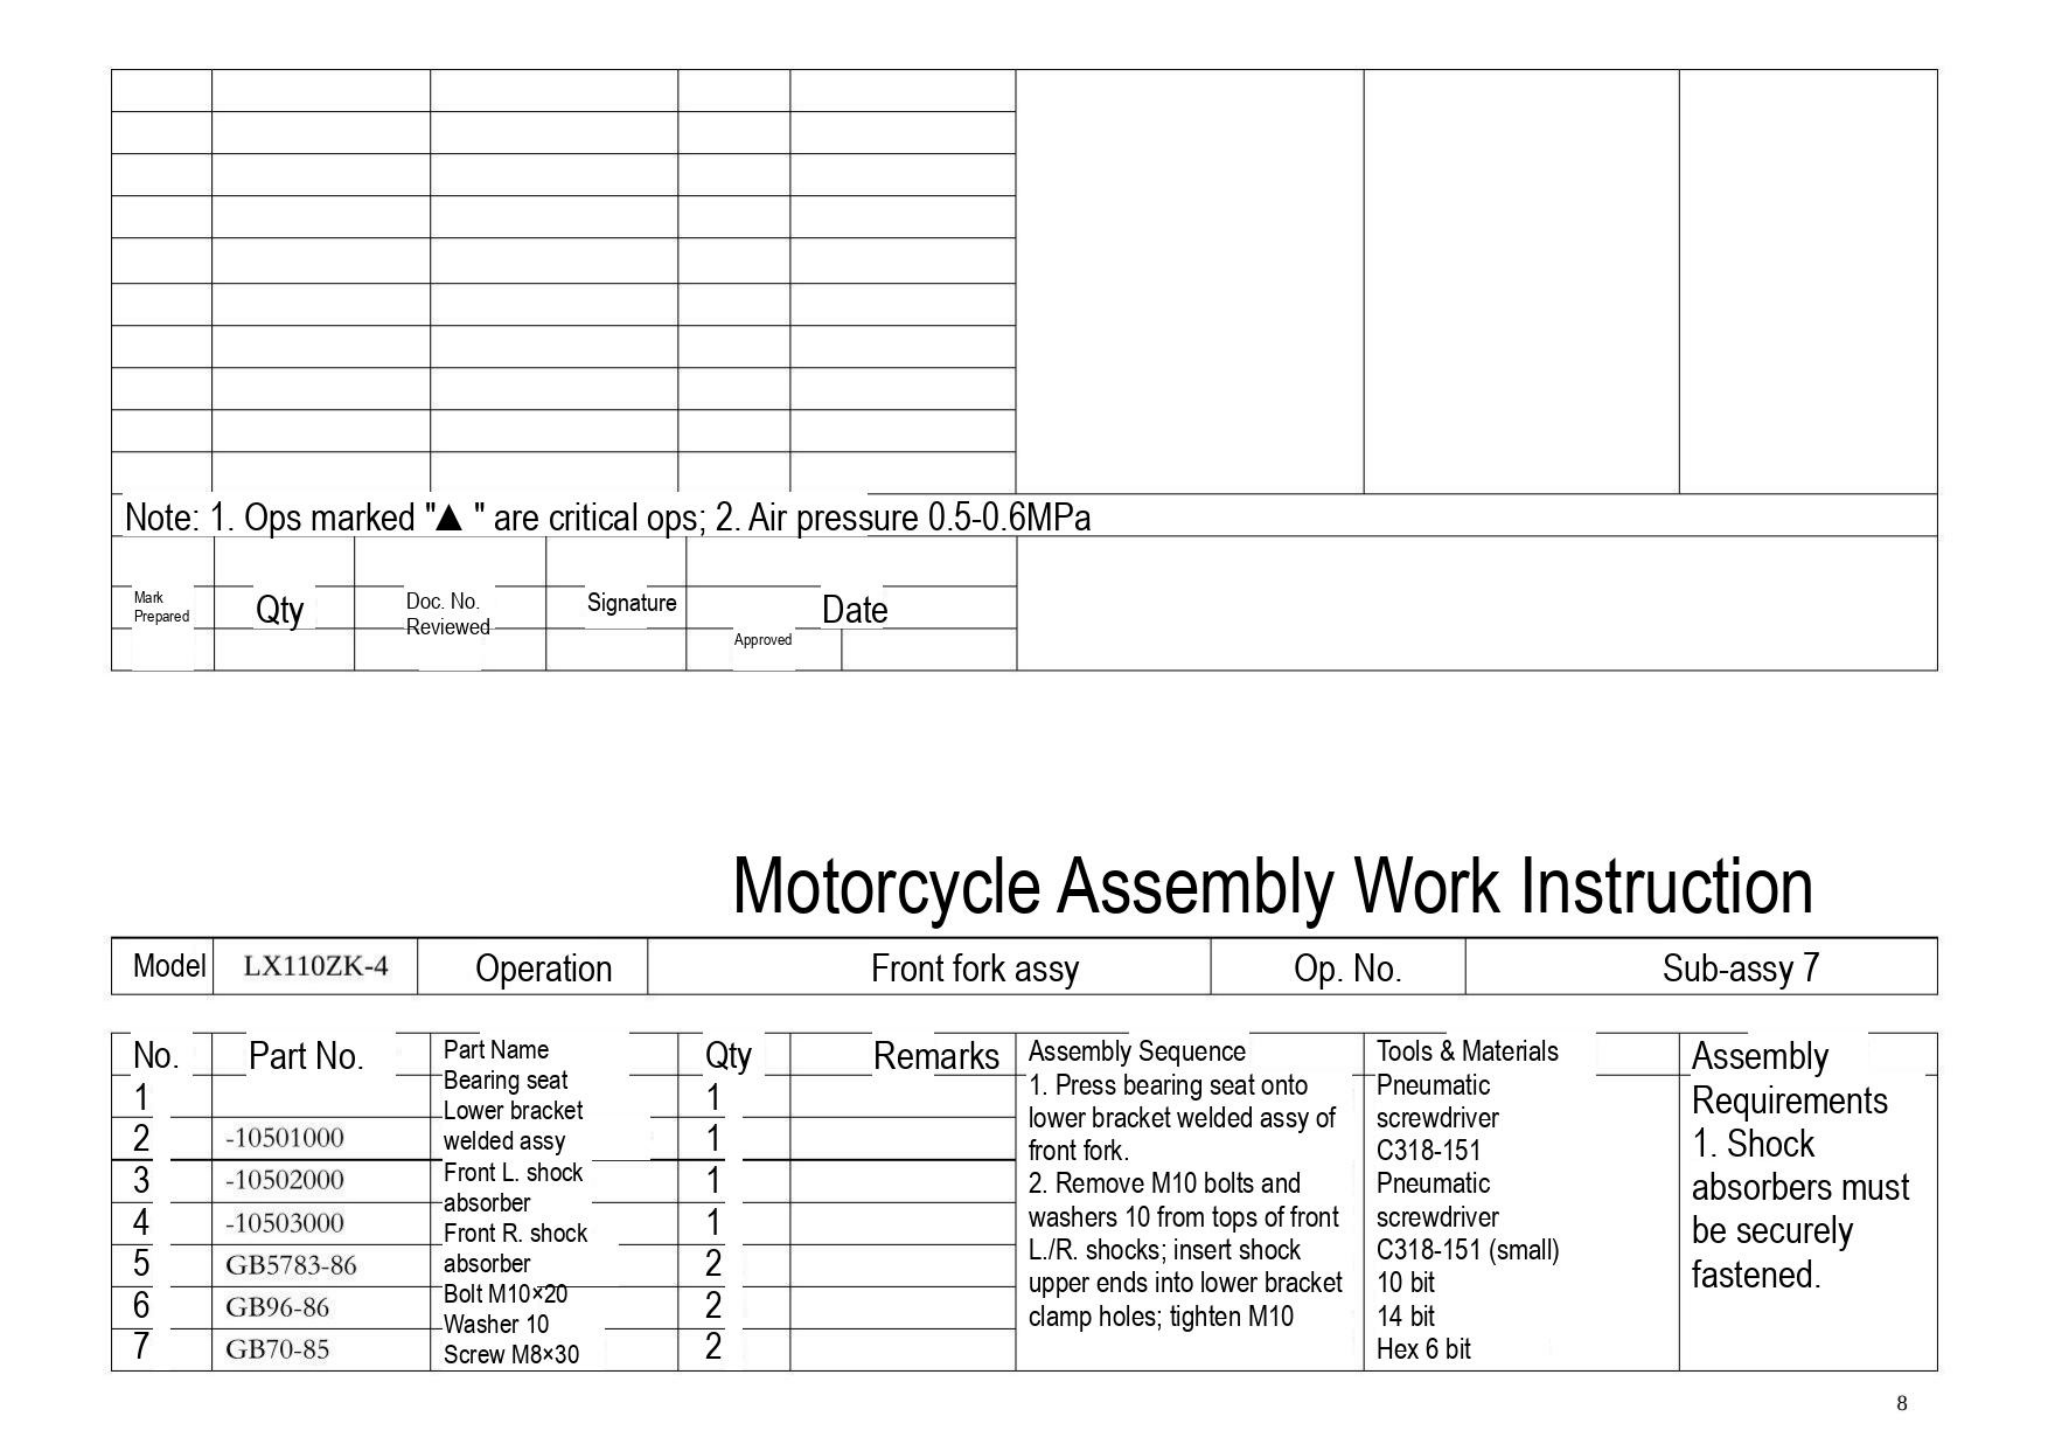Note: 1. Ops marked "▲ " are critical ops; 2. Air pressure 0.5-0.6MPa

| Mark Prepared | Qty | Doc. No. Reviewed | Signature | Approved | Date |
|---|---|---|---|---|---|
| | | | | | |

# Motorcycle Assembly Work Instruction

| Model | LX110ZK-4 | Operation | Front fork assy | Op. No. | Sub-assy 7 |
|---|---|---|---|---|---|

| No. | Part No. | Part Name | Qty | Remarks | Assembly Sequence | Tools & Materials | Assembly Requirements |
|---|---|---|---|---|---|---|---|
| 1 | | Bearing seat | 1 | | 1. Press bearing seat onto lower bracket welded assy of front fork.<br>2. Remove M10 bolts and washers 10 from tops of front L./R. shocks; insert shock upper ends into lower bracket clamp holes; tighten M10 | Pneumatic screwdriver C318-151<br>Pneumatic screwdriver C318-151 (small)<br>10 bit<br>14 bit<br>Hex 6 bit | 1. Shock absorbers must be securely fastened. |
| 2 | -10501000 | Lower bracket welded assy | 1 | | | | |
| 3 | -10502000 | Front L. shock absorber | 1 | | | | |
| 4 | -10503000 | Front R. shock absorber | 1 | | | | |
| 5 | GB5783-86 | Bolt M10×20 | 2 | | | | |
| 6 | GB96-86 | Washer 10 | 2 | | | | |
| 7 | GB70-85 | Screw M8×30 | 2 | | | | |

8
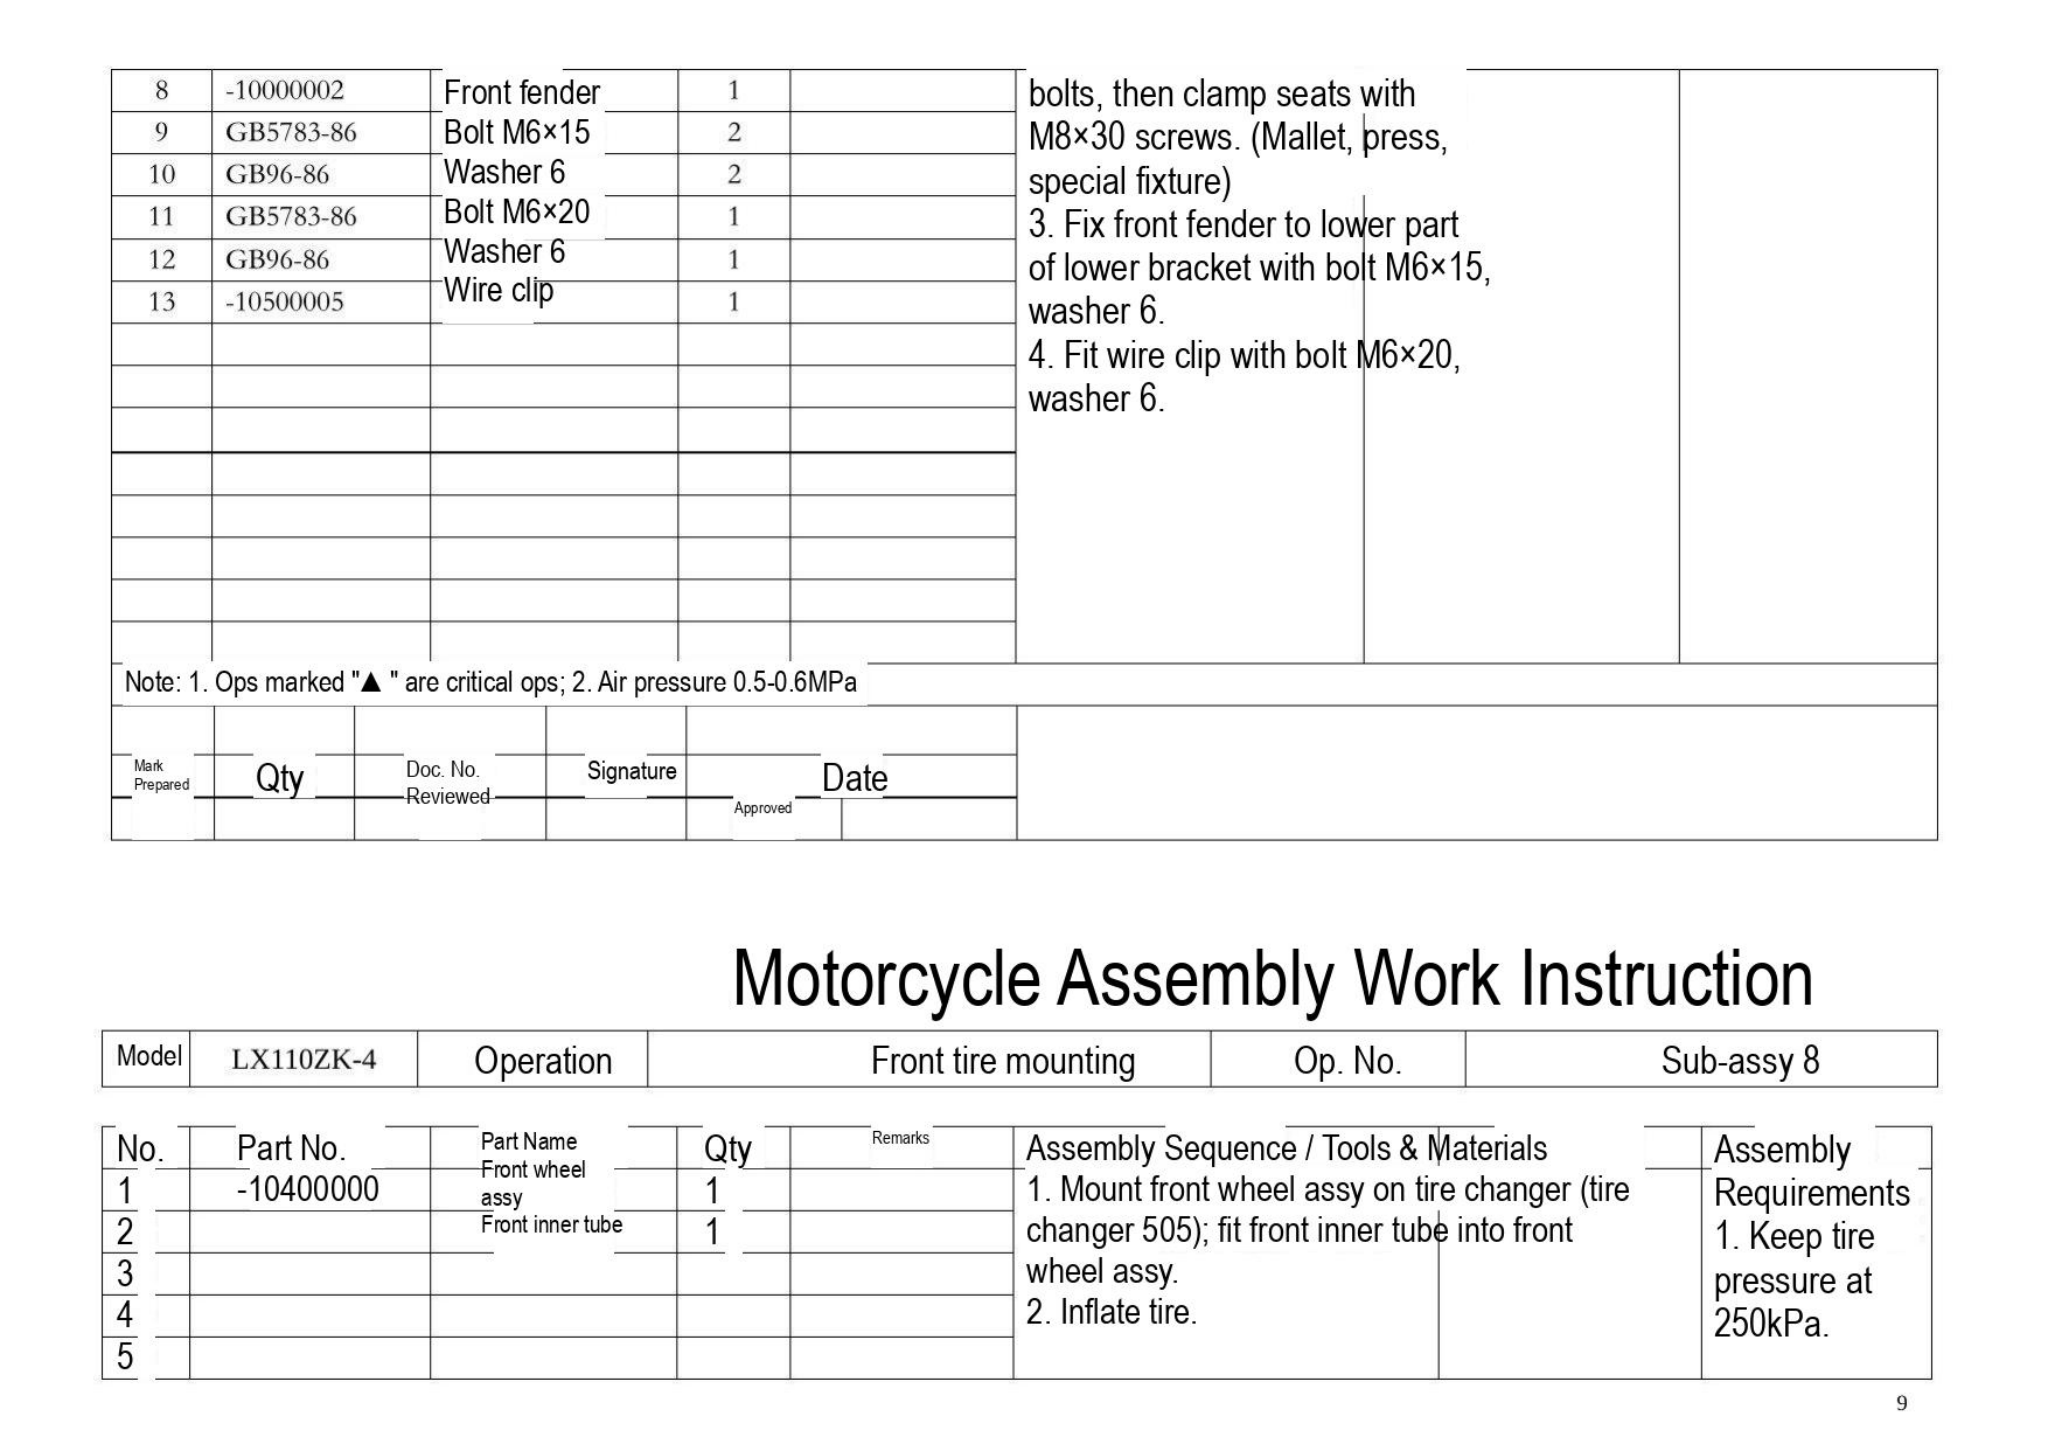| 8 | -10000002 | Front fender | 1 | |
|---|---|---|---|---|
| 9 | GB5783-86 | Bolt M6×15 | 2 | |
| 10 | GB96-86 | Washer 6 | 2 | |
| 11 | GB5783-86 | Bolt M6×20 | 1 | |
| 12 | GB96-86 | Washer 6 | 1 | |
| 13 | -10500005 | Wire clip | 1 | |

bolts, then clamp seats with M8×30 screws. (Mallet, press, special fixture)
3. Fix front fender to lower part of lower bracket with bolt M6×15, washer 6.
4. Fit wire clip with bolt M6×20, washer 6.

Note: 1. Ops marked "▲ " are critical ops; 2. Air pressure 0.5-0.6MPa

| Mark | Qty | Doc. No. | Signature | Date |
|---|---|---|---|---|
| Prepared | | Reviewed | | Approved |

Motorcycle Assembly Work Instruction

| Model | LX110ZK-4 | Operation | Front tire mounting | Op. No. | Sub-assy 8 |
|---|---|---|---|---|---|

| No. | Part No. | Part Name | Qty | Remarks |
|---|---|---|---|---|
| 1 | -10400000 | Front wheel assy | 1 | |
| 2 | | Front inner tube | 1 | |
| 3 | | | | |
| 4 | | | | |
| 5 | | | | |

Assembly Sequence / Tools & Materials
1. Mount front wheel assy on tire changer (tire changer 505); fit front inner tube into front wheel assy.
2. Inflate tire.

Assembly Requirements
1. Keep tire pressure at 250kPa.

9
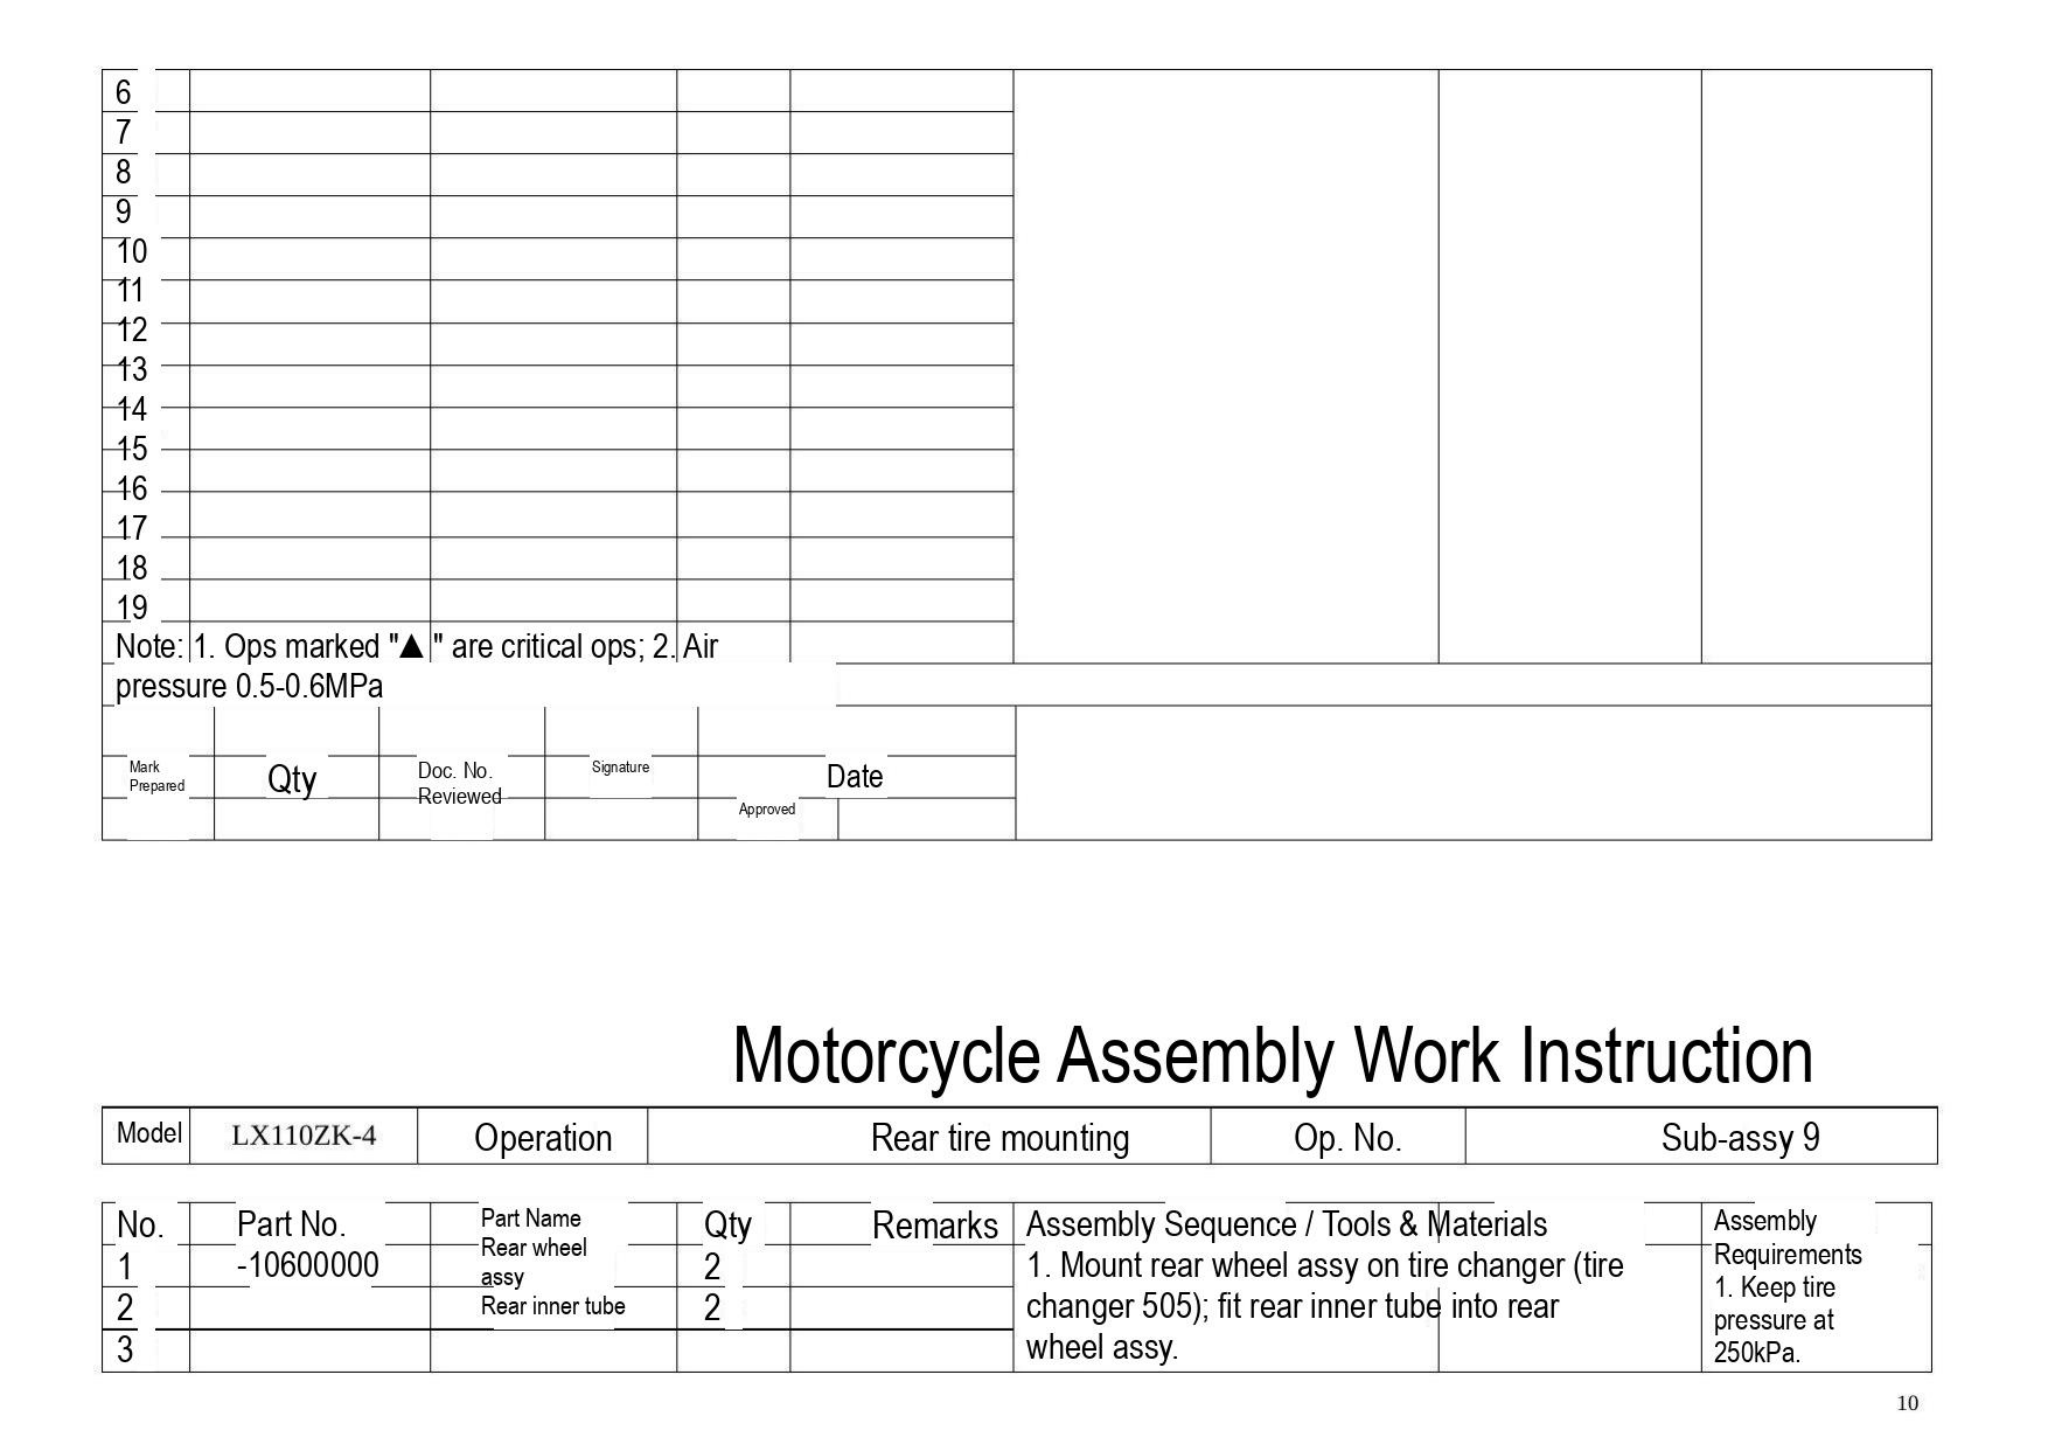| 6 | | | | |
|---|---|---|---|---|
| 7 | | | | |
| 8 | | | | |
| 9 | | | | |
| 10 | | | | |
| 11 | | | | |
| 12 | | | | |
| 13 | | | | |
| 14 | | | | |
| 15 | | | | |
| 16 | | | | |
| 17 | | | | |
| 18 | | | | |
| 19 | | | | |

Note: 1. Ops marked "▲" are critical ops; 2. Air pressure 0.5-0.6MPa

| Mark Prepared | Qty | Doc. No. Reviewed | Signature | Approved | Date |
|---|---|---|---|---|---|
| | | | | | |

# Motorcycle Assembly Work Instruction

| Model | LX110ZK-4 | Operation | Rear tire mounting | Op. No. | Sub-assy 9 |
|---|---|---|---|---|---|

| No. | Part No. | Part Name | Qty | Remarks | Assembly Sequence / Tools & Materials | Assembly Requirements |
|---|---|---|---|---|---|---|
| 1 | -10600000 | Rear wheel assy | 2 | | 1. Mount rear wheel assy on tire changer (tire changer 505); fit rear inner tube into rear wheel assy. | 1. Keep tire pressure at 250kPa. |
| 2 | | Rear inner tube | 2 | | | |
| 3 | | | | | | |

10
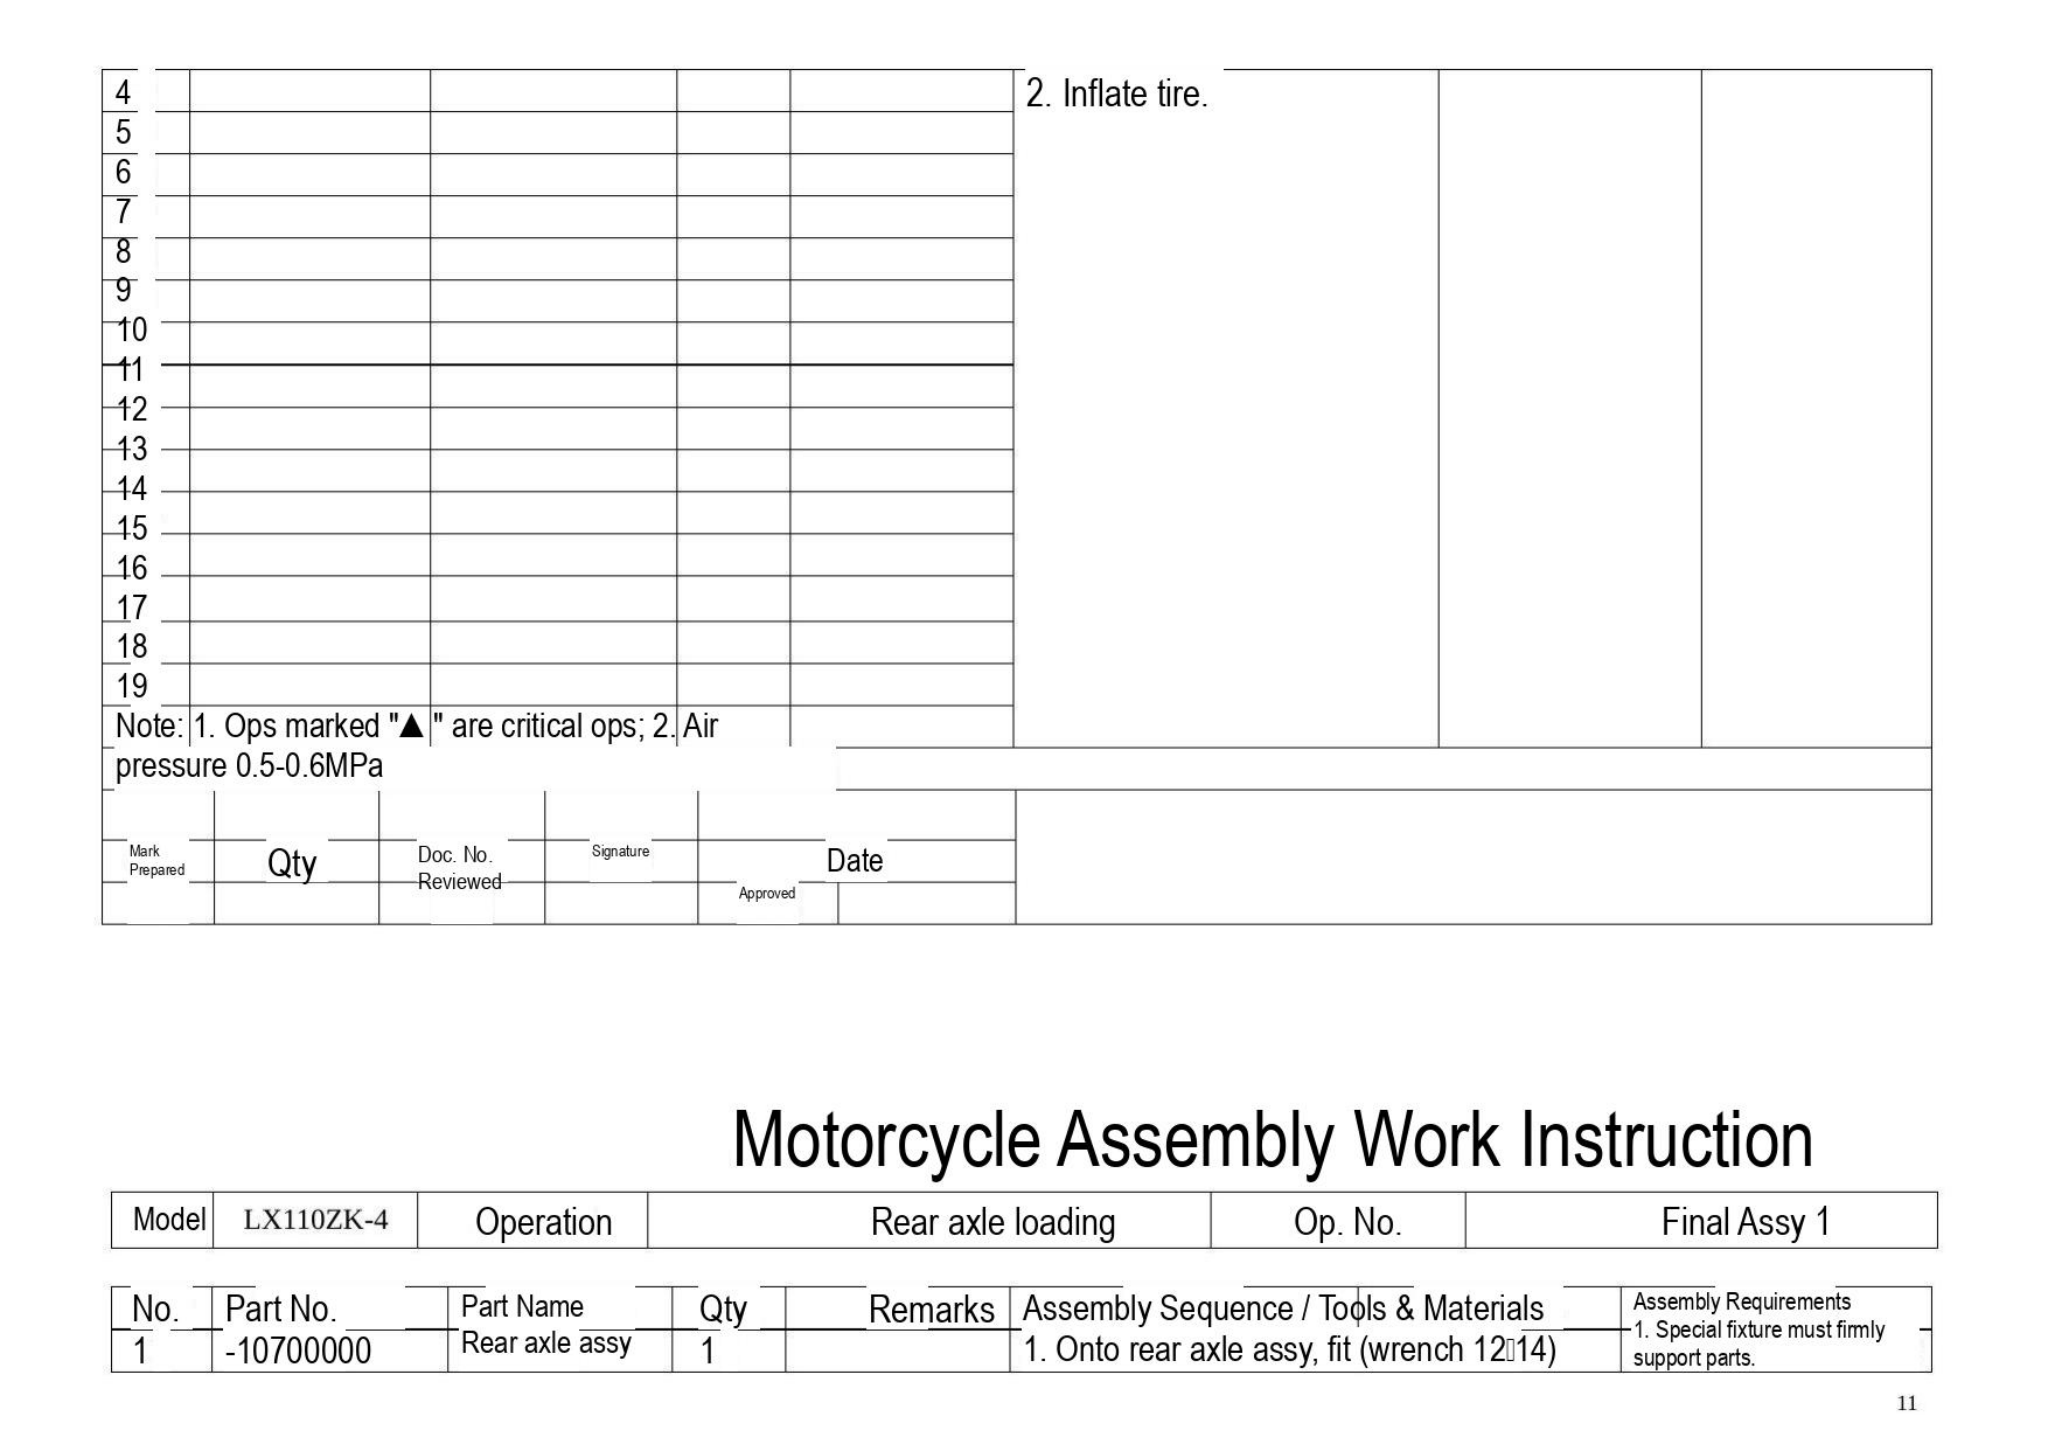|   |   |   |   |   |   |   |   |
|---|---|---|---|---|---|---|---|
| 4 |   |   |   |   | 2. Inflate tire. |   |   |
| 5 |   |   |   |   |   |   |   |
| 6 |   |   |   |   |   |   |   |
| 7 |   |   |   |   |   |   |   |
| 8 |   |   |   |   |   |   |   |
| 9 |   |   |   |   |   |   |   |
| 10 |   |   |   |   |   |   |   |
| 11 |   |   |   |   |   |   |   |
| 12 |   |   |   |   |   |   |   |
| 13 |   |   |   |   |   |   |   |
| 14 |   |   |   |   |   |   |   |
| 15 |   |   |   |   |   |   |   |
| 16 |   |   |   |   |   |   |   |
| 17 |   |   |   |   |   |   |   |
| 18 |   |   |   |   |   |   |   |
| 19 |   |   |   |   |   |   |   |

Note: 1. Ops marked "▲" are critical ops; 2. Air pressure 0.5-0.6MPa

| Mark Prepared | Qty | Doc. No. Reviewed | Signature | Approved | Date |
|---|---|---|---|---|---|
|   |   |   |   |   |   |

# Motorcycle Assembly Work Instruction

| Model | LX110ZK-4 | Operation | Rear axle loading | Op. No. | Final Assy 1 |
|---|---|---|---|---|---|

| No. | Part No. | Part Name | Qty | Remarks | Assembly Sequence / Tools & Materials | Assembly Requirements |
|---|---|---|---|---|---|---|
| 1 | -10700000 | Rear axle assy | 1 |   | 1. Onto rear axle assy, fit (wrench 12 14) | 1. Special fixture must firmly support parts. |

11
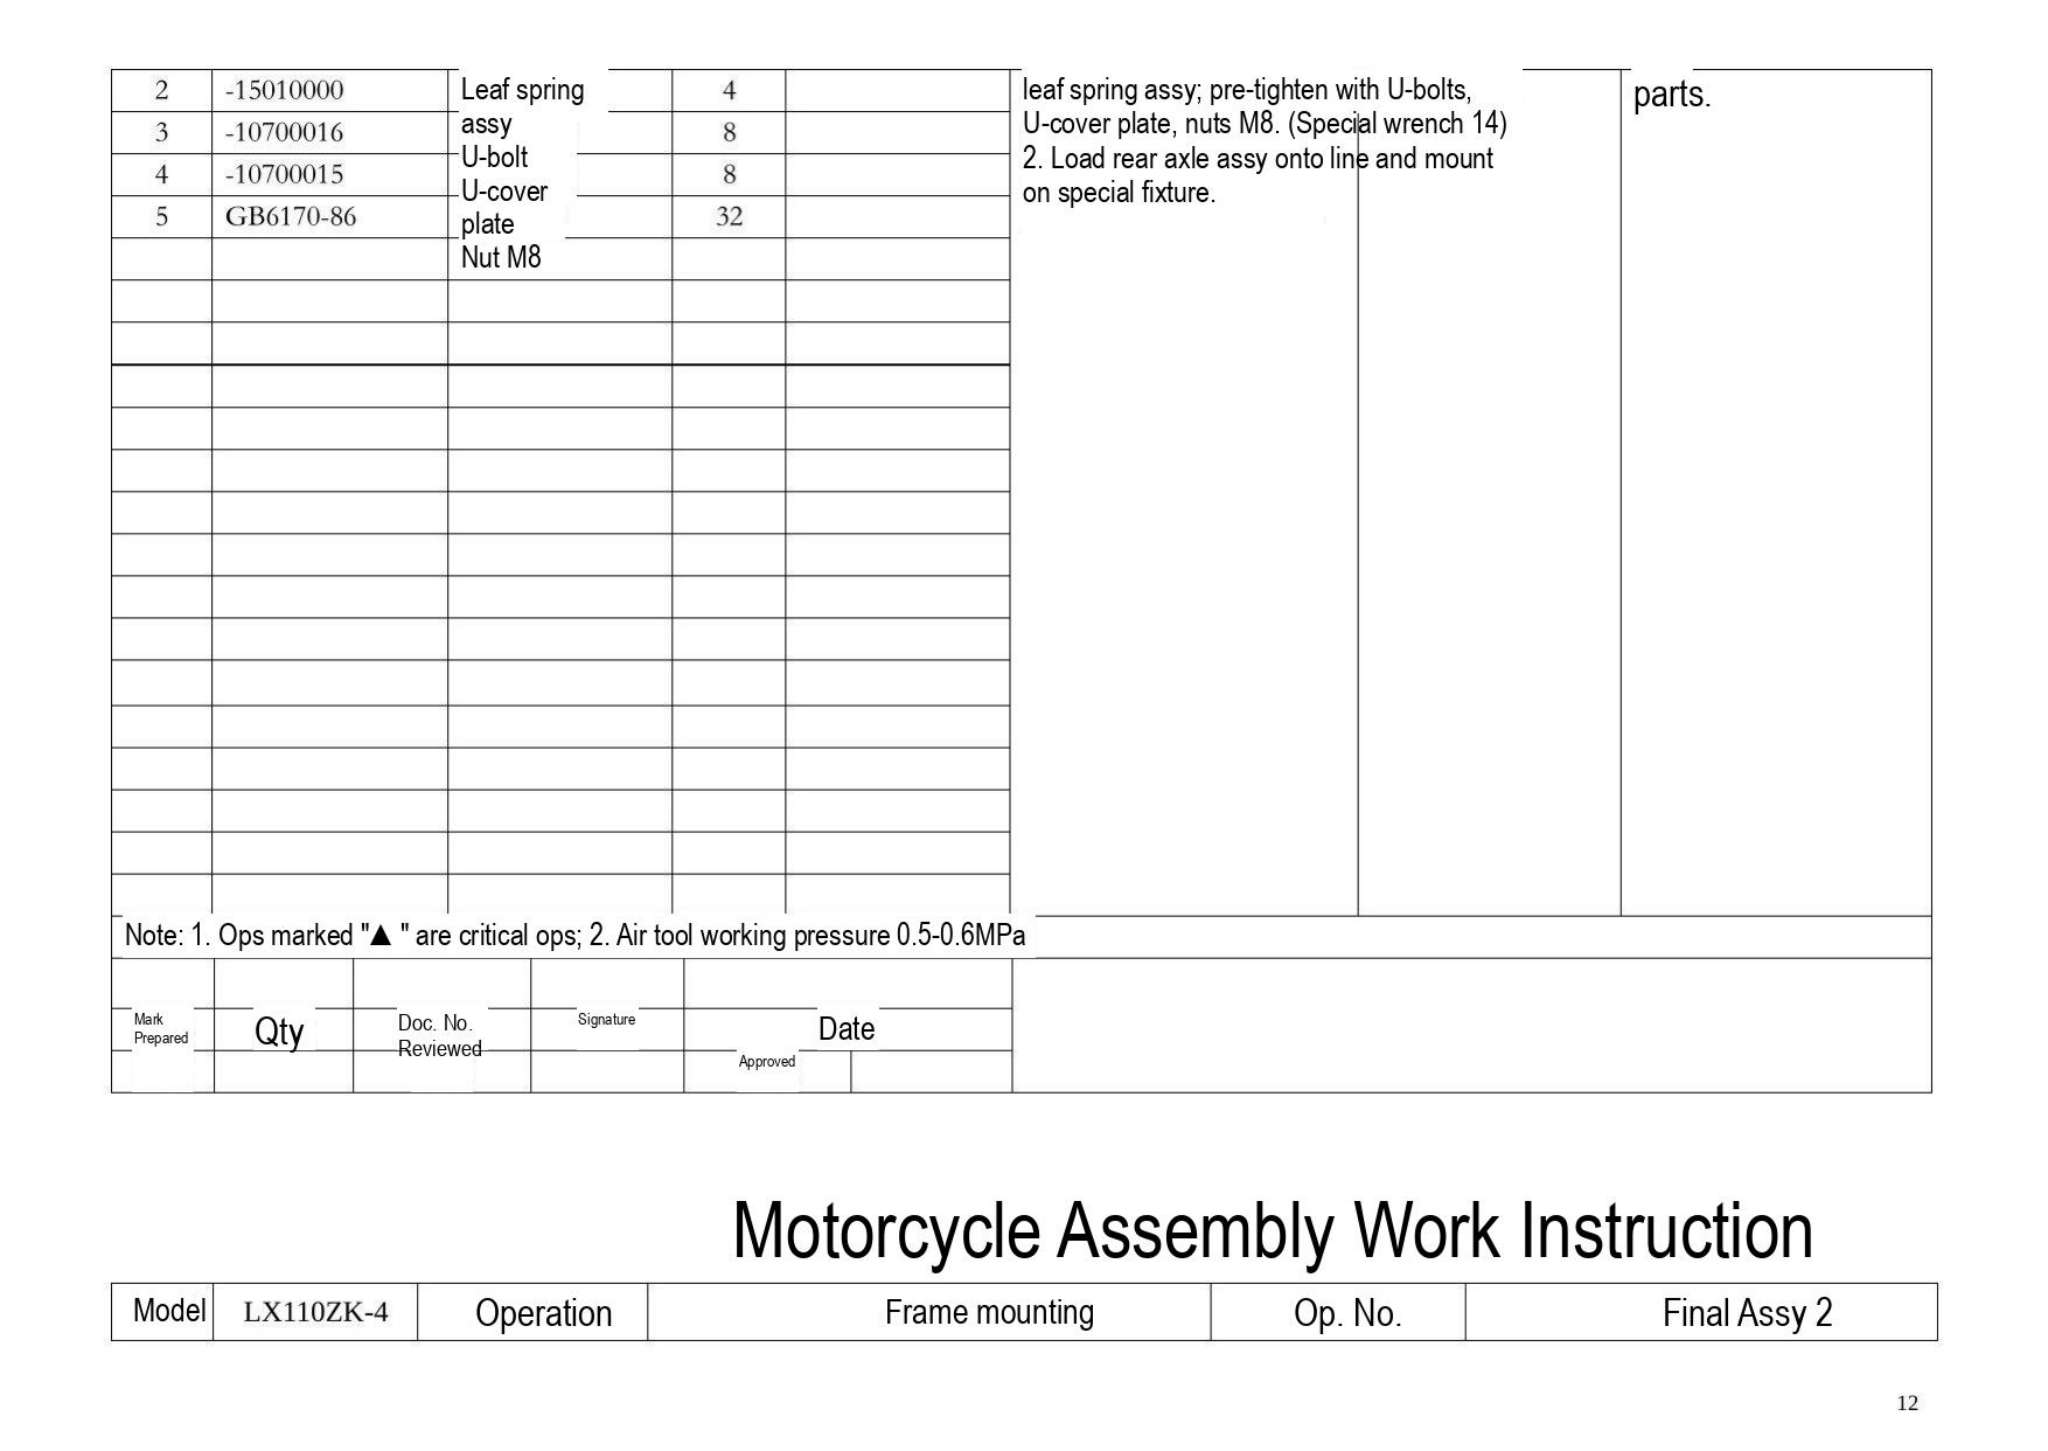| 2 | -15010000 | Leaf spring assy | 4 | | leaf spring assy; pre-tighten with U-bolts, U-cover plate, nuts M8. (Special wrench 14)<br>2. Load rear axle assy onto line and mount on special fixture. | | parts. |
|---|---|---|---|---|---|---|---|
| 3 | -10700016 | U-bolt | 8 | | | | |
| 4 | -10700015 | U-cover plate | 8 | | | | |
| 5 | GB6170-86 | Nut M8 | 32 | | | | |
| | | | | | | | |
| | | | | | | | |
| | | | | | | | |
| | | | | | | | |
| | | | | | | | |
| | | | | | | | |
| | | | | | | | |
| | | | | | | | |
| | | | | | | | |
| | | | | | | | |
| | | | | | | | |
| | | | | | | | |
| | | | | | | | |
| | | | | | | | |
| | | | | | | | |

Note: 1. Ops marked "▲ " are critical ops; 2. Air tool working pressure 0.5-0.6MPa

| Mark<br>Prepared | Qty | Doc. No.<br>Reviewed | Signature | Approved | Date | |
|---|---|---|---|---|---|---|
| | | | | | | |

Motorcycle Assembly Work Instruction

| Model | LX110ZK-4 | Operation | Frame mounting | Op. No. | Final Assy 2 |
|---|---|---|---|---|---|

12
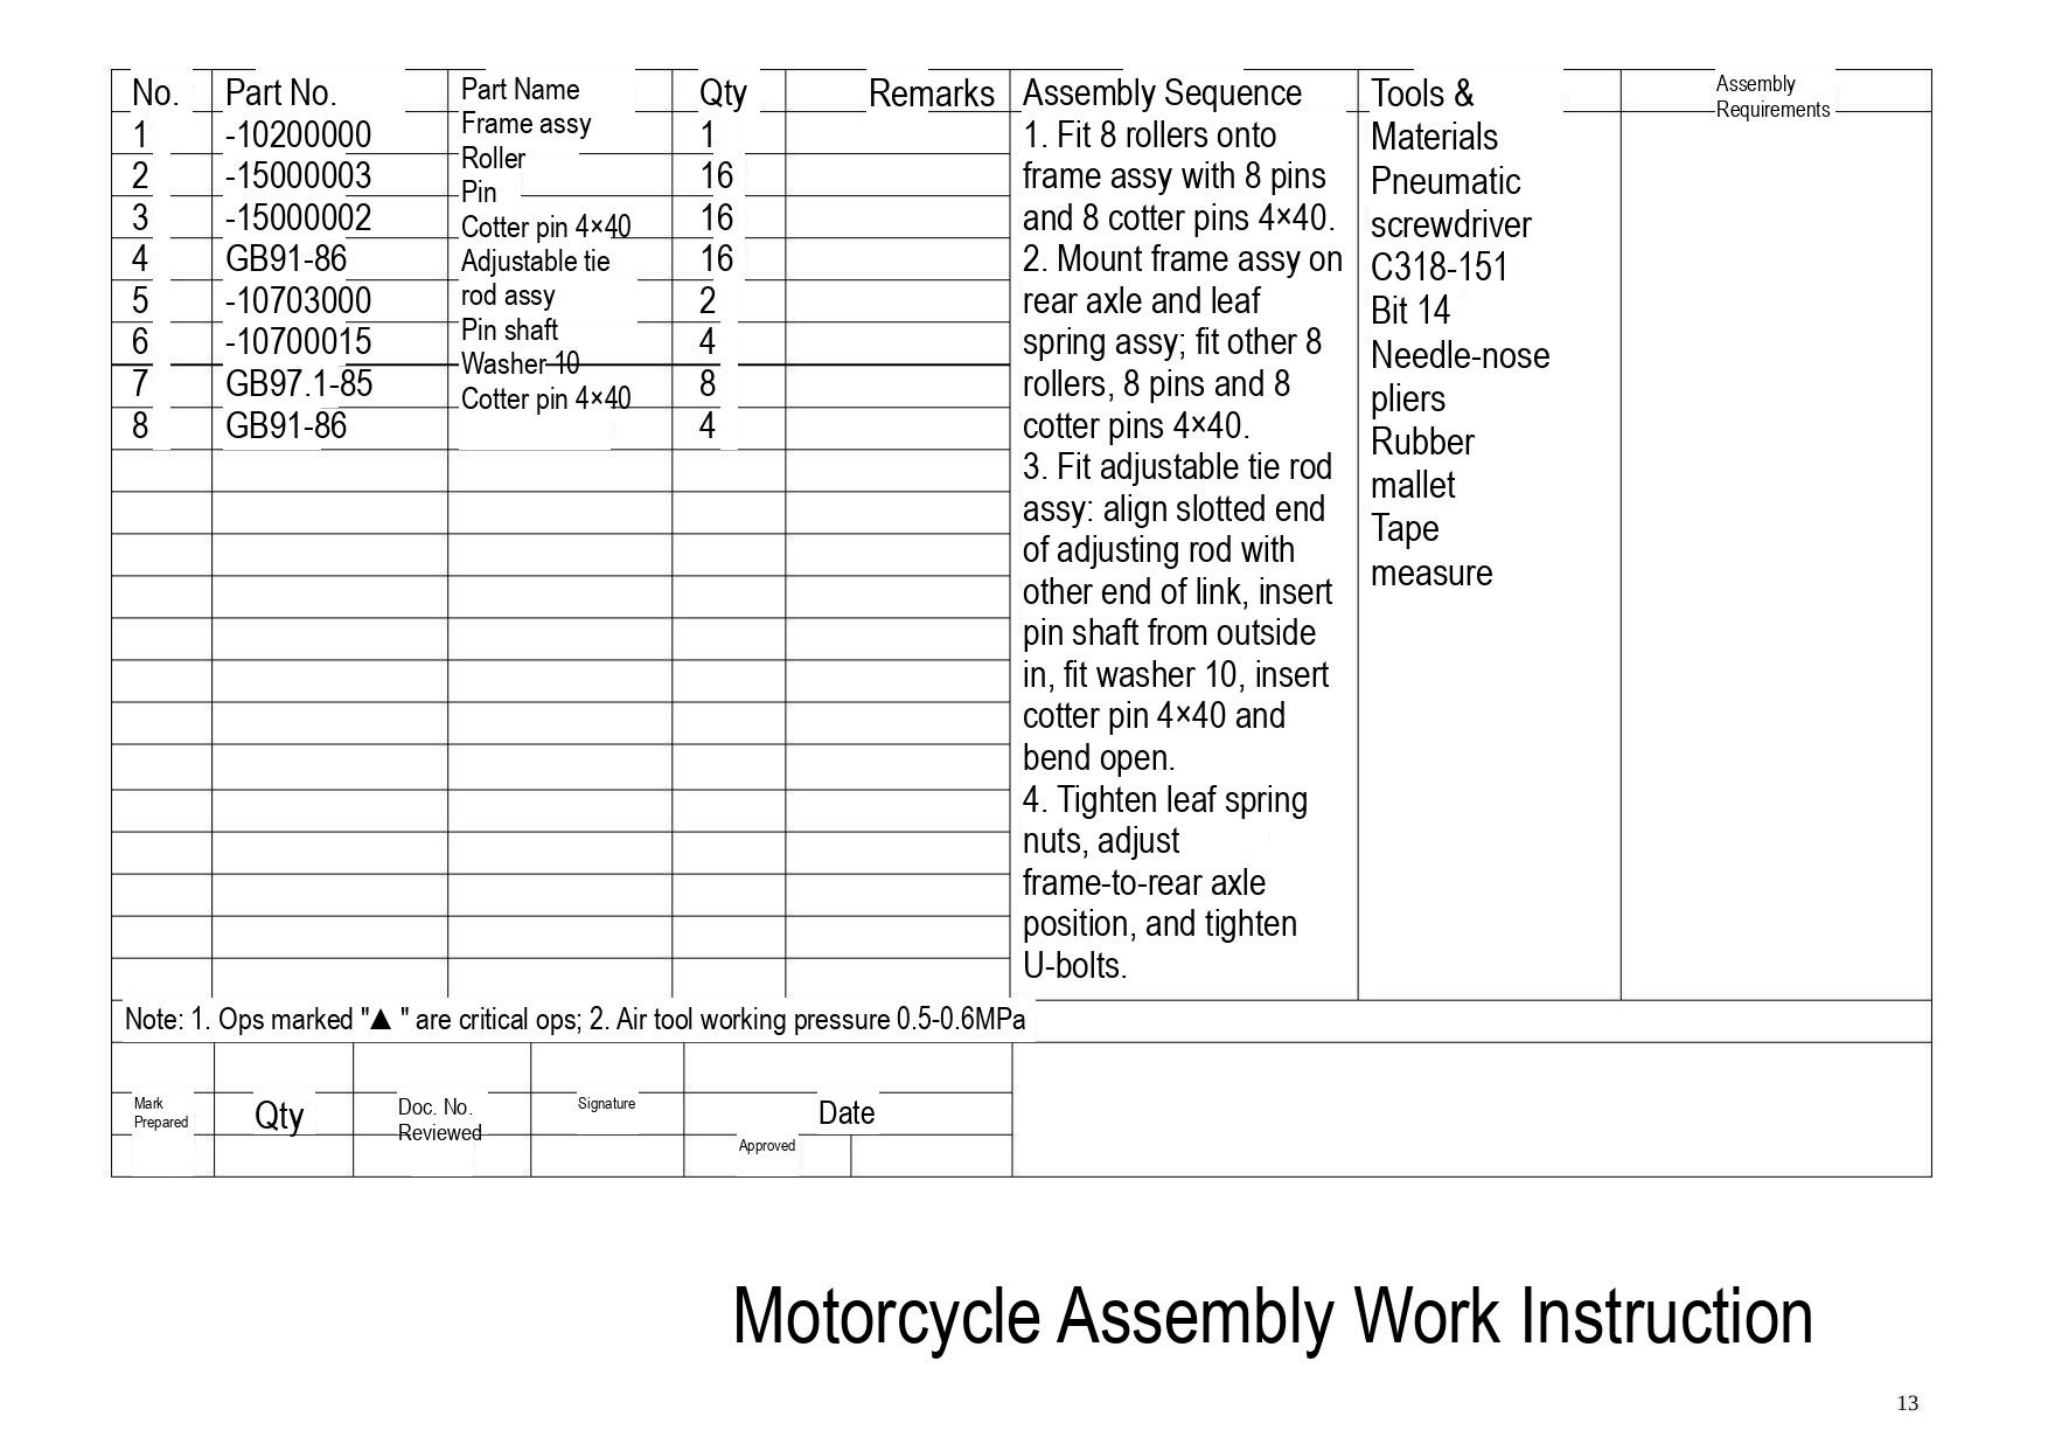| No. | Part No. | Part Name | Qty | Remarks |
|---|---|---|---|---|
| 1 | -10200000 | Frame assy | 1 | |
| 2 | -15000003 | Roller | 16 | |
| 3 | -15000002 | Pin | 16 | |
| 4 | GB91-86 | Cotter pin 4×40 | 16 | |
| 5 | -10703000 | Adjustable tie rod assy | 2 | |
| 6 | -10700015 | Pin shaft | 4 | |
| 7 | GB97.1-85 | Washer 10 | 8 | |
| 8 | GB91-86 | Cotter pin 4×40 | 4 | |

| Assembly Sequence | Tools & Materials | Assembly Requirements |
|---|---|---|
| 1. Fit 8 rollers onto frame assy with 8 pins and 8 cotter pins 4×40.<br>2. Mount frame assy on rear axle and leaf spring assy; fit other 8 rollers, 8 pins and 8 cotter pins 4×40.<br>3. Fit adjustable tie rod assy: align slotted end of adjusting rod with other end of link, insert pin shaft from outside in, fit washer 10, insert cotter pin 4×40 and bend open.<br>4. Tighten leaf spring nuts, adjust frame-to-rear axle position, and tighten U-bolts. | Pneumatic screwdriver C318-151<br>Bit 14<br>Needle-nose pliers<br>Rubber mallet<br>Tape measure | |

Note: 1. Ops marked "▲ " are critical ops; 2. Air tool working pressure 0.5-0.6MPa

| Mark Prepared | Qty | Doc. No. Reviewed | Signature | Approved | Date |
|---|---|---|---|---|---|
| | | | | | |

Motorcycle Assembly Work Instruction

13
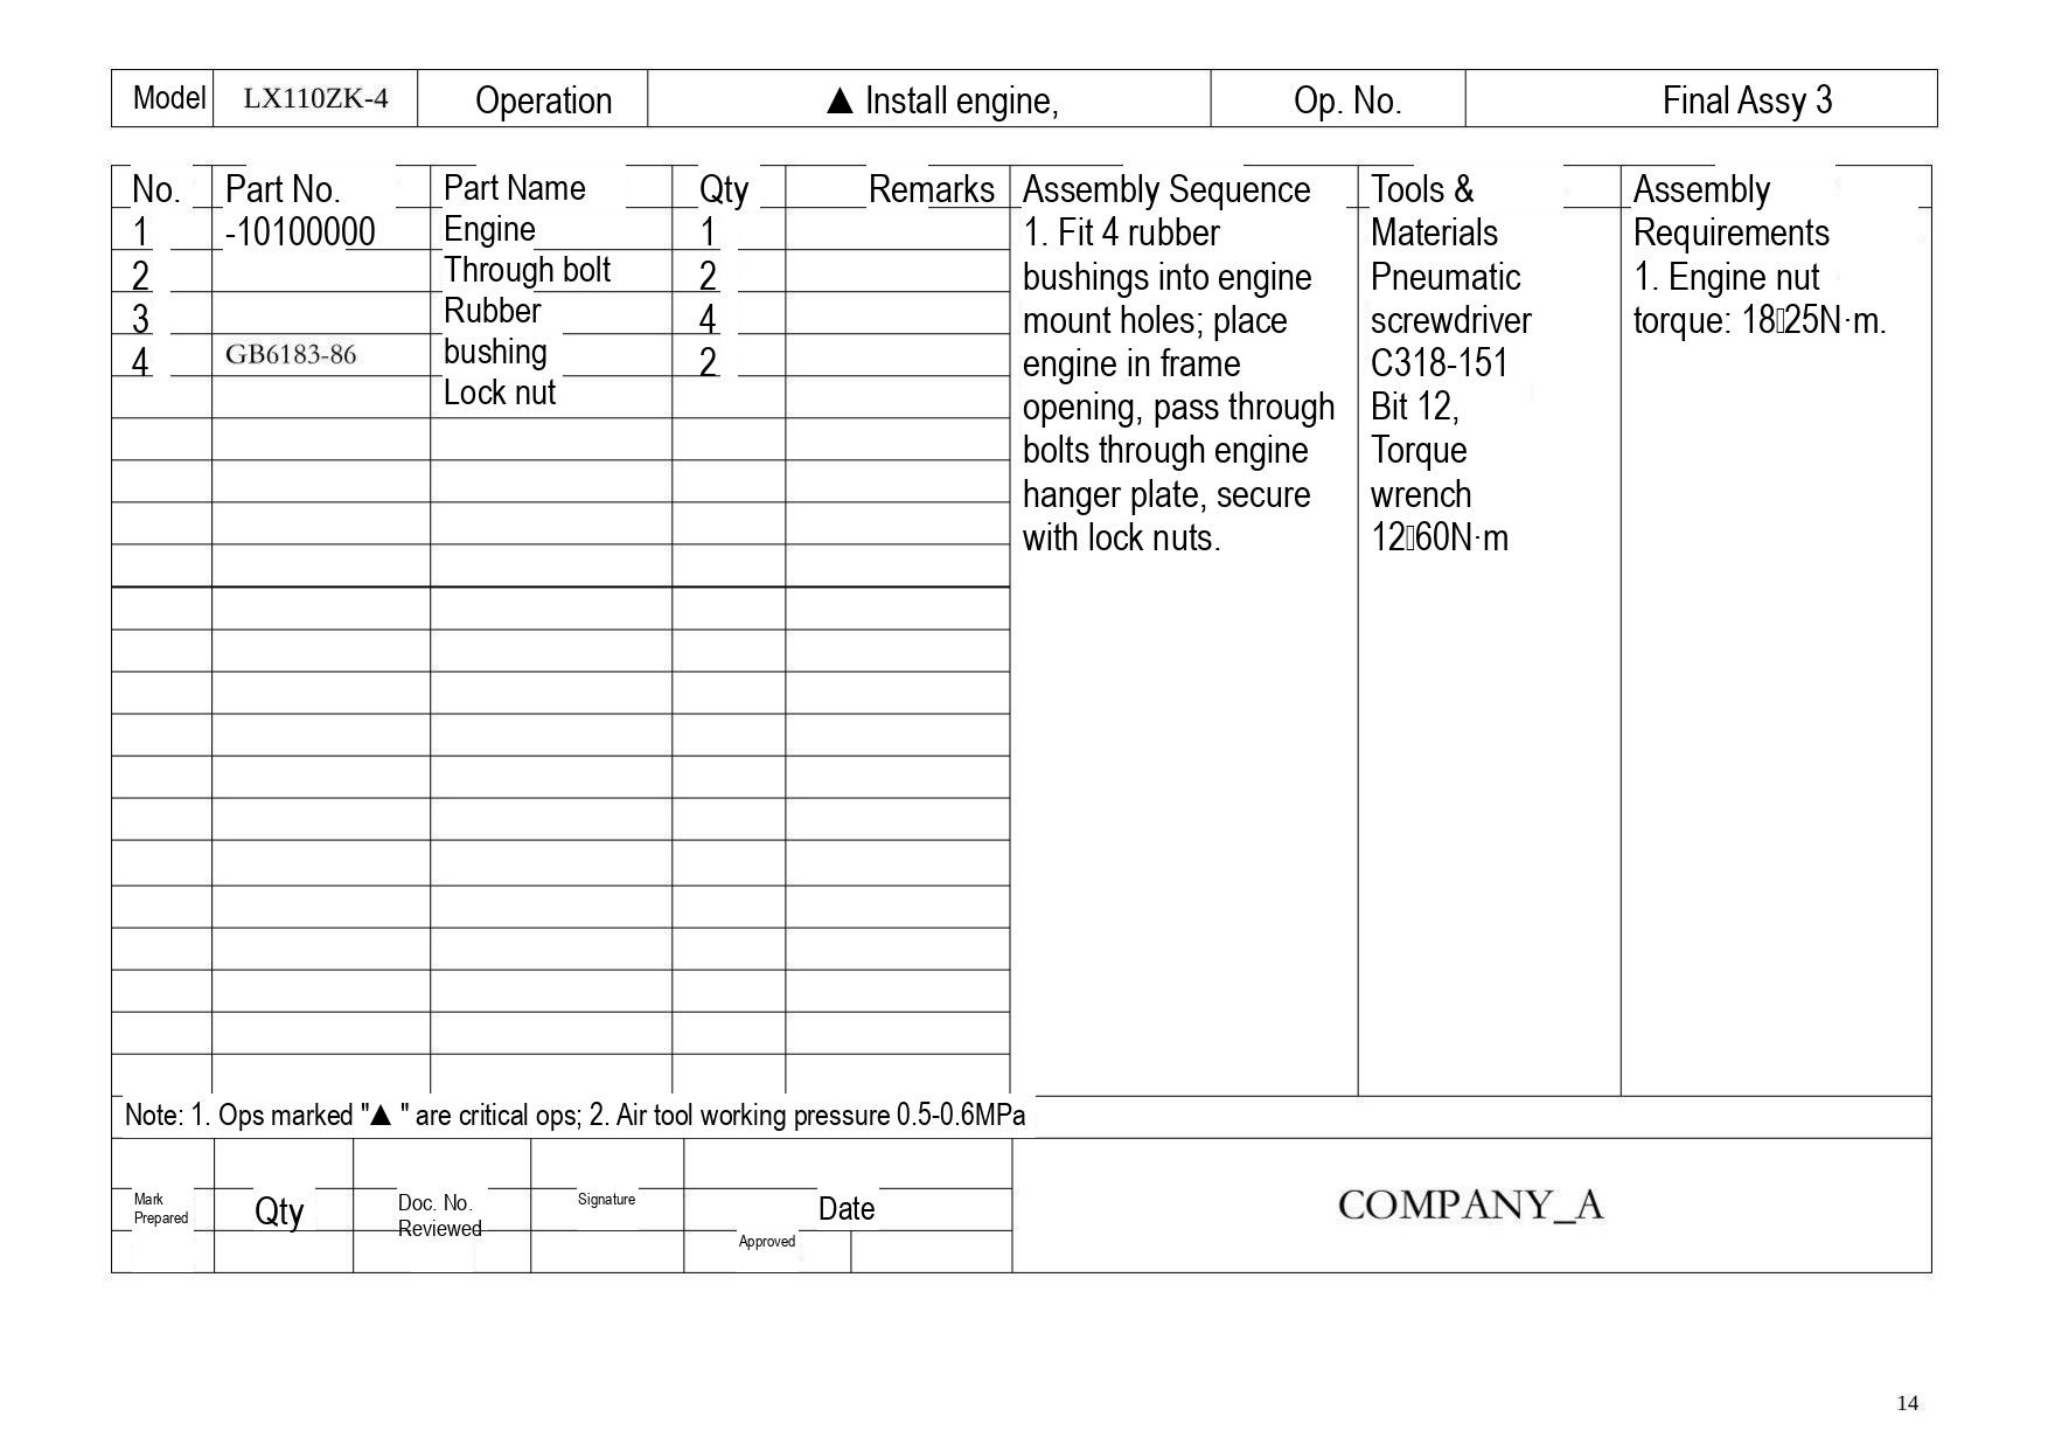| Model | LX110ZK-4 | Operation | ▲ Install engine, | Op. No. | Final Assy 3 |
|---|---|---|---|---|---|

| No. | Part No. | Part Name | Qty | Remarks |
|---|---|---|---|---|
| 1 | -10100000 | Engine | 1 | |
| 2 | | Through bolt | 2 | |
| 3 | | Rubber | 4 | |
| 4 | GB6183-86 | bushing | 2 | |
| | | Lock nut | | |

| Assembly Sequence | Tools & Materials | Assembly Requirements |
|---|---|---|
| 1. Fit 4 rubber bushings into engine mount holes; place engine in frame opening, pass through bolts through engine hanger plate, secure with lock nuts. | Pneumatic screwdriver C318-151 Bit 12, Torque wrench 12▯60N·m | 1. Engine nut torque: 18▯25N·m. |

Note: 1. Ops marked "▲ " are critical ops; 2. Air tool working pressure 0.5-0.6MPa

| Mark | Qty | Doc. No. | Signature | Date | COMPANY_A |
|---|---|---|---|---|---|
| Prepared | | Reviewed | | Approved | |

14